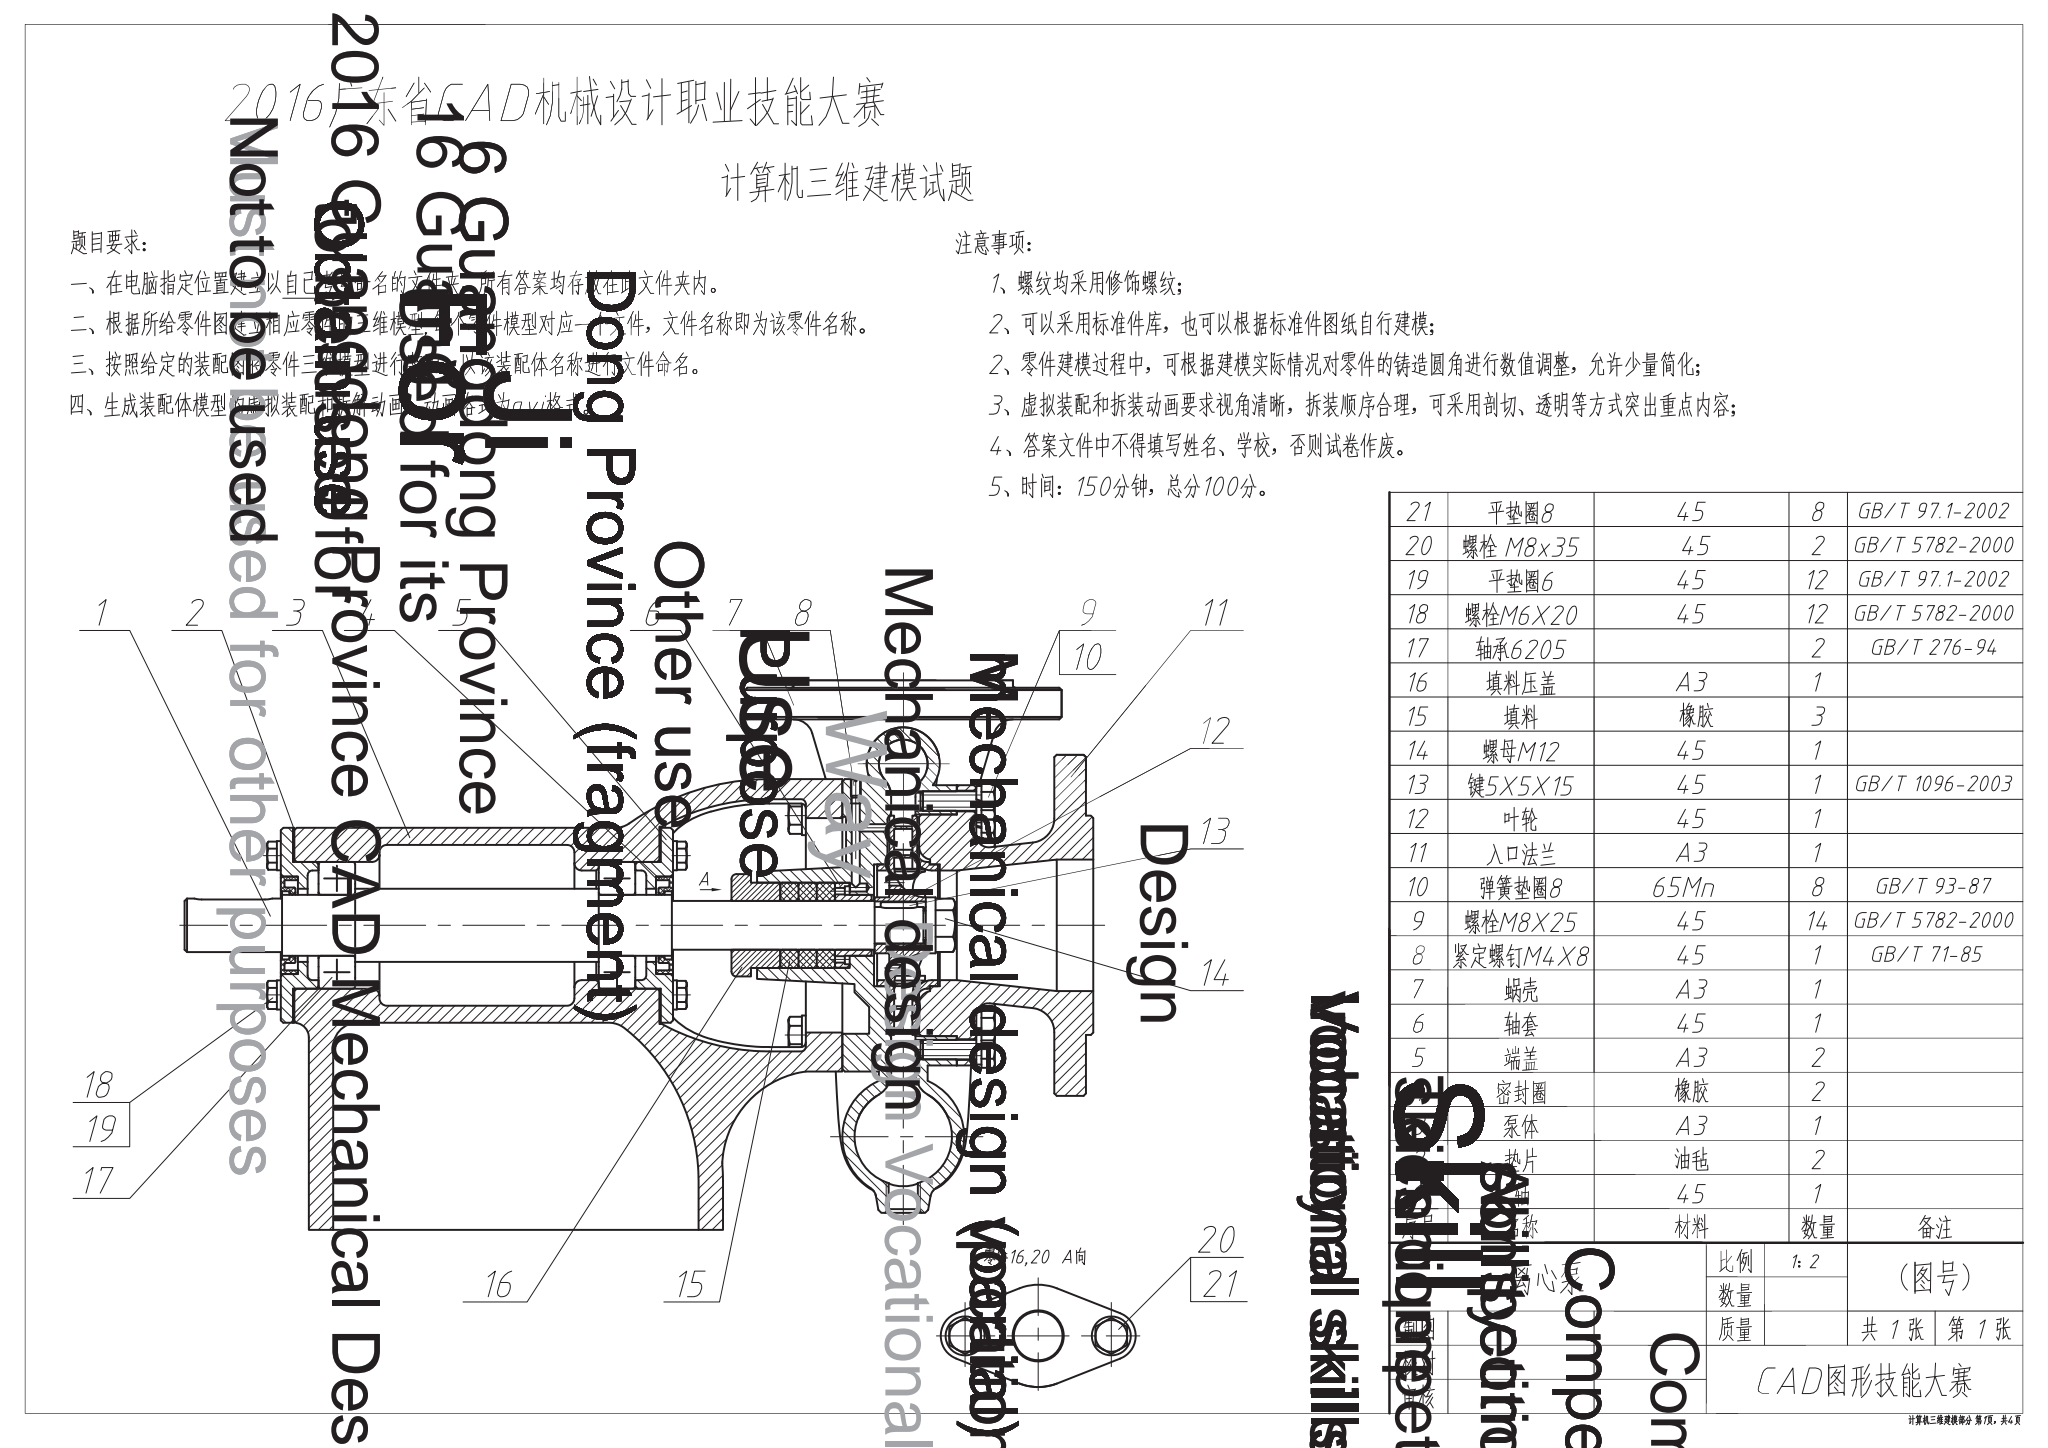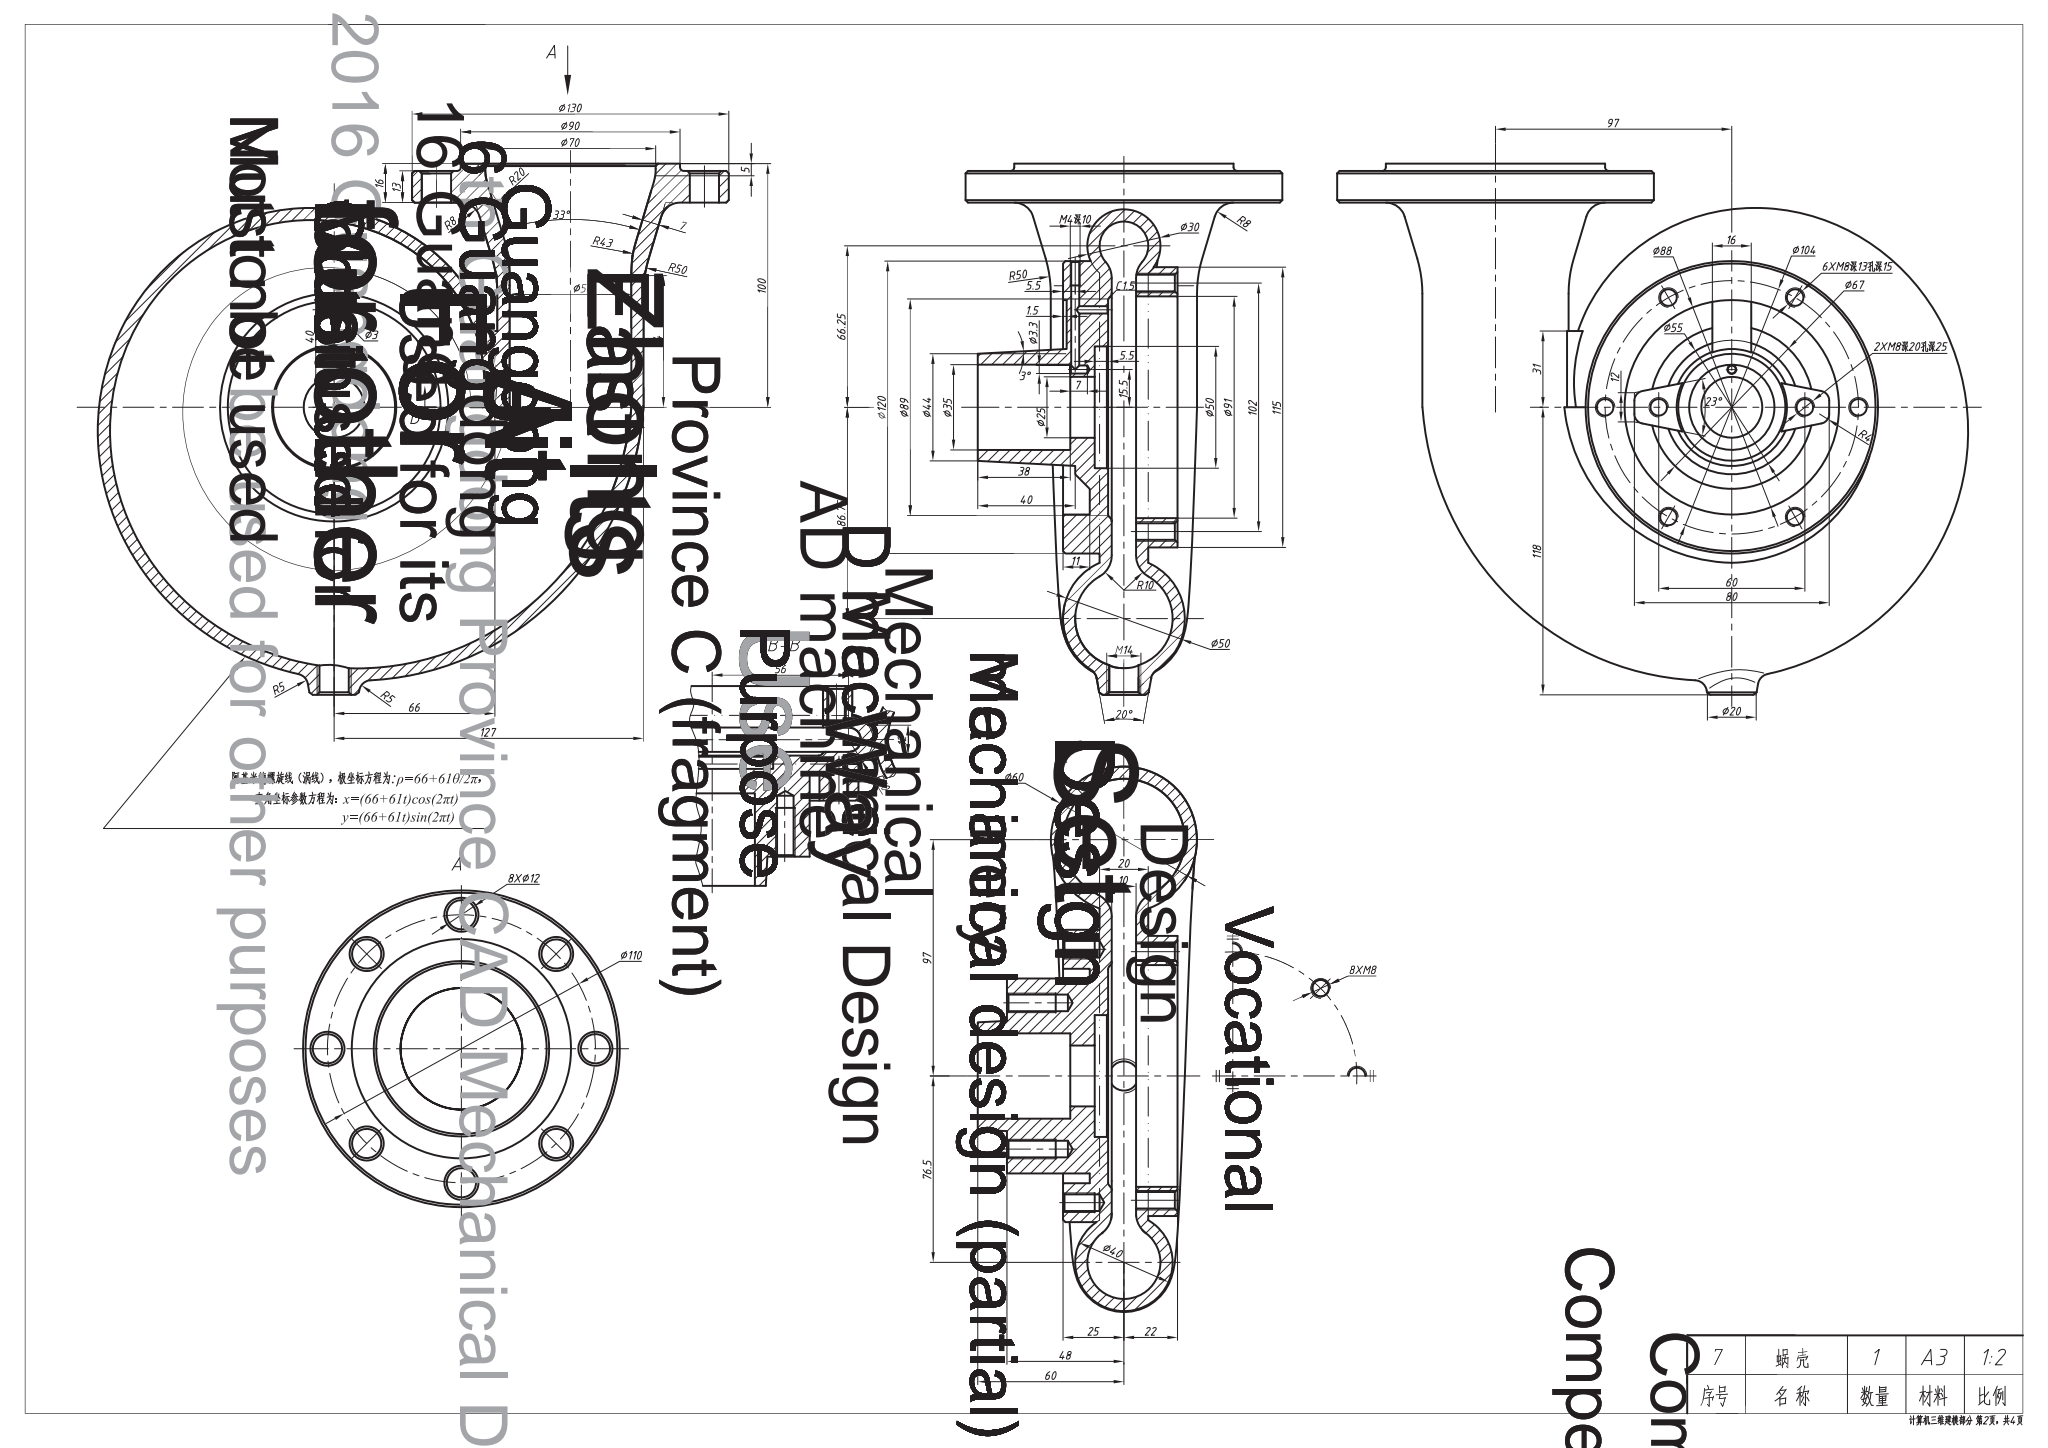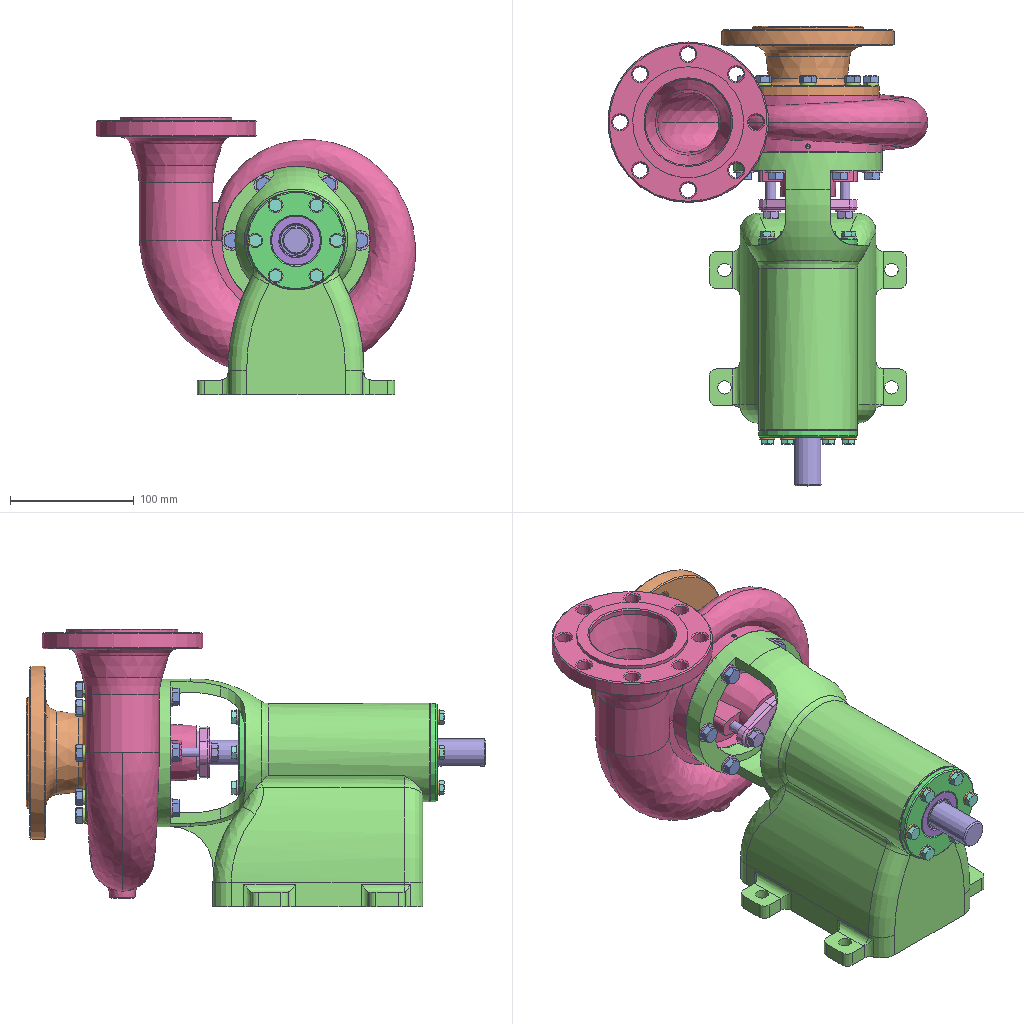Assembly | NX | 21 different items | 77 placed | box 259 x 372 x 225 mm
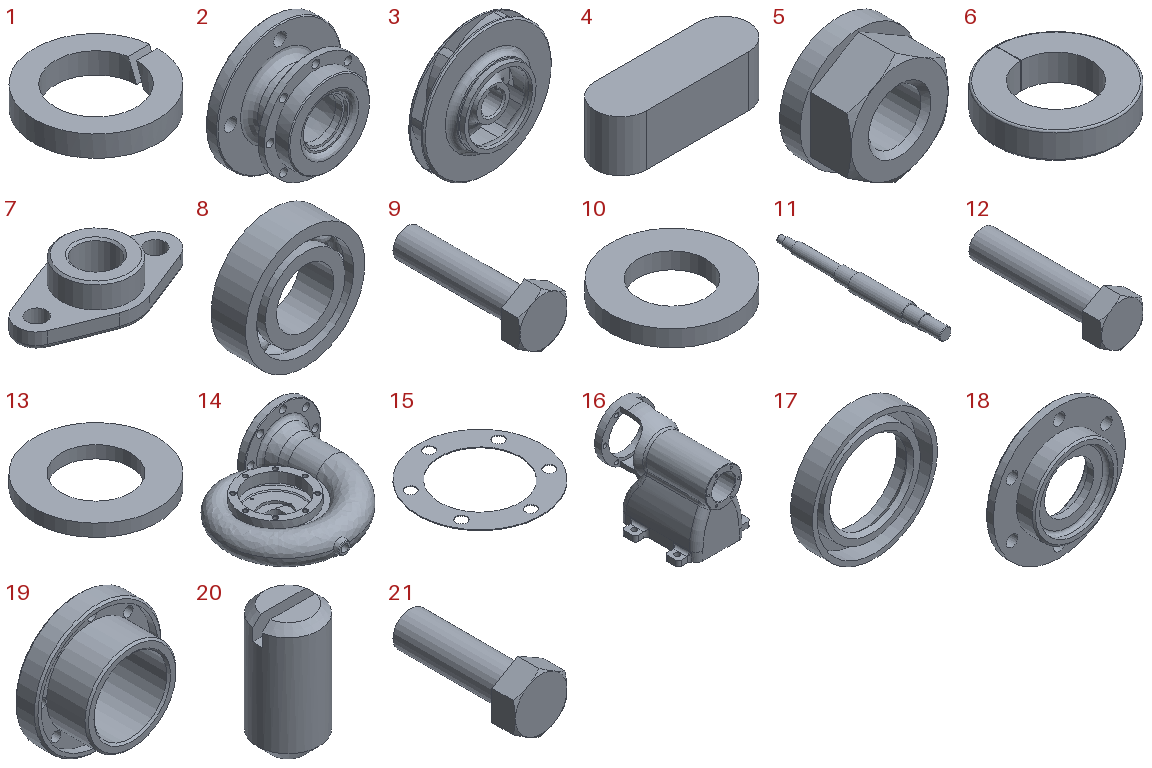Parts list (item | quantity | size | volume | features):
1 | x8 | 12.3 x 12.3 x 2.1 mm | 137.929 mm3 | features DATUM_CSYS 3, EXTRUDE 2, SKETCH 2
2 | x1 | 140 x 71.5 x 140 mm | 362768 mm3 | features DATUM_CSYS 4, SKETCH 3, EXTRUDE 2, BLEND 1, CHAMFER 1, SWP104 1
3 | x1 | 90 x 26 x 90 mm | 37267 mm3 | features DATUM_CSYS 5, SKETCH 4, EXTRUDE 3, CHAMFER 1, REPLACE_FACE 1, SWP104 1, UNITE 1
4 | x1 | 15 x 5 x 5 mm | 348.175 mm3 | features DATUM_CSYS 2, EXTRUDE 1, SKETCH 1
5 | x1 | 23 x 12 x 23 mm | 3134 mm3 | features DATUM_CSYS 4, SKETCH 3, CHAMFER 2, EXTRUDE 2, HOLE PACKAGE 1, SIMPLE HOLE 1, SWP104 1, SYMBOLIC_THREAD 1
6 | x3 | 35 x 35 x 7.5 mm | 4837 mm3 | features DATUM_CSYS 2, BLEND 1, EXTRUDE 1, SKETCH 1
7 | x1 | 80 x 42 x 20 mm | 22097 mm3 | features DATUM_CSYS 3, EXTRUDE 2, SKETCH 2, BLEND 1, CHAMFER 1, REPLACE_FACE 1
8 | x2 | 52 x 15 x 52 mm | 17377 mm3 | features SPHERE 8, Instance Feature 7, DATUM_CSYS 2, Pattern Feature 1, SKETCH 1, SWP104 1
9 | x12 | 10 x 29 x 11.547 mm | 1052 mm3 | features DATUM_CSYS 4, SKETCH 3, EXTRUDE 2, SWP104 1, SYMBOLIC_THREAD 1, UNITE 1
10 | x12 | 12 x 12 x 1.6 mm | 126.217 mm3 | features DATUM_CSYS 2, EXTRUDE 1, SKETCH 1
11 | x1 | 30 x 315.25 x 30 mm | 145532 mm3 | features DATUM_CSYS 4, SKETCH 3, DATUM_PLANE 2, EXTRUDE 2, CHAMFER 1, SWP104 1, SYMBOLIC_THREAD 1
12 | x2 | 12 x 40.5 x 13.856 mm | 2443 mm3 | features DATUM_CSYS 4, SKETCH 3, EXTRUDE 2, SWP104 1, SYMBOLIC_THREAD 1, UNITE 1
13 | x8 | 16 x 16 x 1.6 mm | 219.911 mm3 | features DATUM_CSYS 2, EXTRUDE 1, SKETCH 1
14 | x1 | 258.983 x 218 x 130 mm | 729840 mm3 | features DATUM_CSYS 27, SKETCH 26, SIMPLE HOLE 22, SYMBOLIC_THREAD 18, EXTRUDE 17, REPLACE_FACE 15, UNITE 10, HOLE PACKAGE 9, TRIM BODY 7, CHAMFER 6, ASSOCIATIVE_INTERSECTION 5, BLEND 3, OFFSET_REGION 3, CPROJ 2, Container 2, DRAFT 2, EXTRACT_BODY 2, Geometry Instance 2, SWP104 2, DATUM_PLANE 1, SHELL 1, SKIN 1, SPLINE_LAW 1
15 | x2 | 80 x 80 x 0.5 mm | 1336 mm3 | features DATUM_CSYS 2, EXTRUDE 1, SKETCH 1
16 | x1 | 160 x 225 x 185 mm | 973073 mm3 | features DATUM_CSYS 25, SKETCH 24, EXTRACT_DATUM_AXIS 18, EXTRACT_FACE 18, HOLE PACKAGE 18, SIMPLE HOLE 18, Instance Feature 15, SYMBOLIC_THREAD 12, EXTRUDE 11, REPLACE_FACE 10, BLEND 8, UNITE 7, OFFSET_REGION 4, Pattern Feature 3, CHAMFER 1, CPROJ 1, Container 1, EXTRACT_BODY 1, Geometry Instance 1, SWP104 1, TRIM BODY 1
17 | x2 | 40 x 7 x 40 mm | 2796 mm3 | features DATUM_CSYS 2, SKETCH 1, SWP104 1
18 | x2 | 80 x 15.5 x 80 mm | 27346 mm3 | features DATUM_CSYS 3, SKETCH 2, EXTRUDE 1, SWP104 1
19 | x1 | 34.8 x 15 x 34.8 mm | 4556 mm3 | features DATUM_CSYS 3, SKETCH 2, EXTRUDE 1, SWP104 1
20 | x1 | 4 x 4 x 8 mm | 90.888 mm3 | features DATUM_CSYS 3, CHAMFER 2, SKETCH 2, EXTRUDE 1, SWP104 1, SYMBOLIC_THREAD 1
21 | x14 | 12 x 30.5 x 13.856 mm | 1941 mm3 | features DATUM_CSYS 4, SKETCH 3, EXTRUDE 2, SWP104 1, SYMBOLIC_THREAD 1, UNITE 1
Mates (type | each side: item.copy, entity, surface, feature):
Fix | 16.1 component
Touch | 15.1 face plane Extrude(1) | 16.1 face plane Revolve(1)
Touch | 15.1 face cylinder Extrude(1) | 16.1 face cylinder Pattern Feature [Circular] (49) / Instance[4][0]
Touch | 15.1 face cylinder Extrude(1) | 16.1 face cylinder Revolve(1)
Touch | 18.1 face plane Revolve(1) | 15.1 face plane Extrude(1) | 2 times
Touch | 18.1 face cylinder Extrude(2) | 15.1 edge
Touch | 18.1 face cylinder Revolve(1) | 16.1 face cylinder Revolve(1) | 2 times
Touch | 17.1 face plane Revolve(1) | 18.1 face plane Revolve(1)
Touch | 18.1 face cylinder Revolve(1) | 17.1 face cylinder Revolve(1)
Touch | 17.1 face cylinder Revolve(1) | 18.1 face cylinder Revolve(1) | 2 times
Touch | 18.1 face cylinder Extrude(2) | 16.1 face cylinder Pattern Feature [Circular] (53) / Instance[1][0]
Touch | 8.1 face plane Revolve(1) | 11.1 face plane Revolve(1) | 2 times
Touch | 11.1 face cylinder Revolve(1) | 8.1 face cylinder Revolve(1)
Touch | 8.1 face cylinder Revolve(1) | 11.1 face cylinder Revolve(1)
Touch | 2.1 face cylinder Revolve(1) | 14.1 face cylinder Ø91 Hole(49)
Touch | 14.1 face cylinder M8 x 1.25 Threaded Hole(83) | 2.1 face cylinder Extrude(3)
Touch | 14.1 face plane Trim Body(46) | 2.1 face plane Revolve(1)
Touch | 8.1 face plane Revolve(1) | 18.1 face plane Revolve(1)
Touch | 11.1 face cylinder Revolve(1) | 16.1 face cylinder Revolve(1)
Touch | 18.1 face plane Revolve(1) | 17.1 face plane Revolve(1)
Touch | 3.1 face cylinder Revolve(1) | 2.1 face cylinder Revolve(1)
Touch | 3.1 face plane Revolve(1) | 2.1 face plane Revolve(1)
Touch | 11.1 face cylinder Revolve(1) | 3.1 face cylinder Revolve(1)
Parallel | 11.1 face plane Extrude(4) | 3.1 face plane Extrude(6)
Touch | 4.1 face plane Extrude(1) | 11.1 face plane Extrude(4) | 2 times
Touch | 4.1 face cylinder Extrude(1) | 11.1 face cylinder Extrude(4)
Touch | 3.1 face plane Revolve(1) | 11.1 face plane Revolve(1)
Touch | 5.1 face cylinder M12 x 1.75 Threaded Hole(4) | 2.1 face cylinder Revolve(1)
Touch | 5.1 face plane Extrude(2) | 3.1 face plane Revolve(1)
Touch | 20.1 face cylinder Revolve(1) | 14.1 face cylinder M4 x 0.7 Threaded Hole(79)
Touch | 14.1 face cylinder Extrude(44) | 20.1 face plane Revolve(1)
Touch | 16.1 face cylinder Pattern Feature [Circular] (51) / Instance[1][0] | 14.1 face cylinder M8 x 1.25 Threaded Hole(76)
Touch | 19.1 face plane Revolve(1) | 14.1 face plane Ø35 Hole(57)
Touch | 19.1 face cylinder Revolve(1) | 14.1 face cylinder Ø35 Hole(57)
Touch | 6.1 face plane Extrude(1) | 6.1 face plane Extrude(1) | 2 times
Touch | 6.1 face cylinder Extrude(1) | 6.1 face cylinder Extrude(1) | 2 times
Touch | 6.1 face plane Extrude(1) | 19.1 face plane Revolve(1)
Touch | 14.1 face cylinder Ø35 Hole(57) | 6.1 face cylinder Extrude(1)
Touch | 7.1 face plane Extrude(2) | 6.1 face plane Extrude(1)
Touch | 14.1 face cylinder Ø35 Hole(57) | 7.1 face cylinder Extrude(2)
Touch | 7.1 face cylinder Extrude(1) | 14.1 face cylinder M8 x 1.25 Threaded Hole(75)
Touch | 10.1 face plane Extrude(1) | 18.1 face plane Revolve(1) | 2 times
Touch | 10.1 face cylinder Extrude(1) | 18.1 face cylinder Extrude(2)
Touch | 10.1 face plane Extrude(1) | 9.1 face plane Extrude(1) | 2 times
Touch | 9.1 face cylinder Extrude(3) | 10.1 face cylinder Extrude(1)
Touch | 10.1 face cylinder Extrude(1) | 9.1 face cylinder Extrude(3)
Touch | 9.1 face cylinder Extrude(3) | 18.1 face cylinder Extrude(2)
Touch | 1.1 face plane Extrude(1) | 21.1 face plane Extrude(1)
Touch | 1.1 face cylinder Extrude(1) | 21.1 face cylinder Extrude(3)
Touch | 1.1 face plane Extrude(1) | 2.1 face plane Revolve(1)
Touch | 2.1 face cylinder Extrude(3) | 21.1 face cylinder Extrude(3)
Touch | 13.1 face plane Extrude(1) | 12.1 face plane Extrude(1)
Touch | 12.1 face cylinder Extrude(3) | 13.1 face cylinder Extrude(1)
Touch | 13.1 face plane Extrude(1) | 7.1 face plane Extrude(1)
Touch | 7.1 face cylinder Extrude(1) | 12.1 face cylinder Extrude(3)
Touch | 16.1 face plane Revolve(1) | 13.1 face plane Extrude(1)
Touch | 21.1 face cylinder Extrude(3) | 16.1 face cylinder Pattern Feature [Circular] (51) / Instance[1][0]
Bond | 16.1 component | assembly component | 2 times
Bond | 10.1 component | assembly component | 12 times
Bond | 9.1 component | assembly component | 12 times
CircularPattern | assembly axis | assembly csys | assembly csys | assembly csys | assembly csys | assembly csys | assembly csys | 6 times
Bond | 21.1 component | assembly component | 14 times
Bond | 13.1 component | assembly component | 6 times
Bond | 2.1 component | assembly component
Bond | 1.1 component | assembly component | 8 times
CircularPattern | assembly axis | assembly csys | assembly csys | assembly csys | assembly csys | assembly csys | assembly csys | assembly csys | assembly csys | 2 times
Touch | 16.1 face plane Revolve(1) | 15.1 face plane Extrude(1)
Touch | 15.1 face cylinder Extrude(1) | 9.1 face cylinder Extrude(3)
Touch | 15.1 face cylinder Extrude(1) | 18.1 face cylinder Revolve(1)